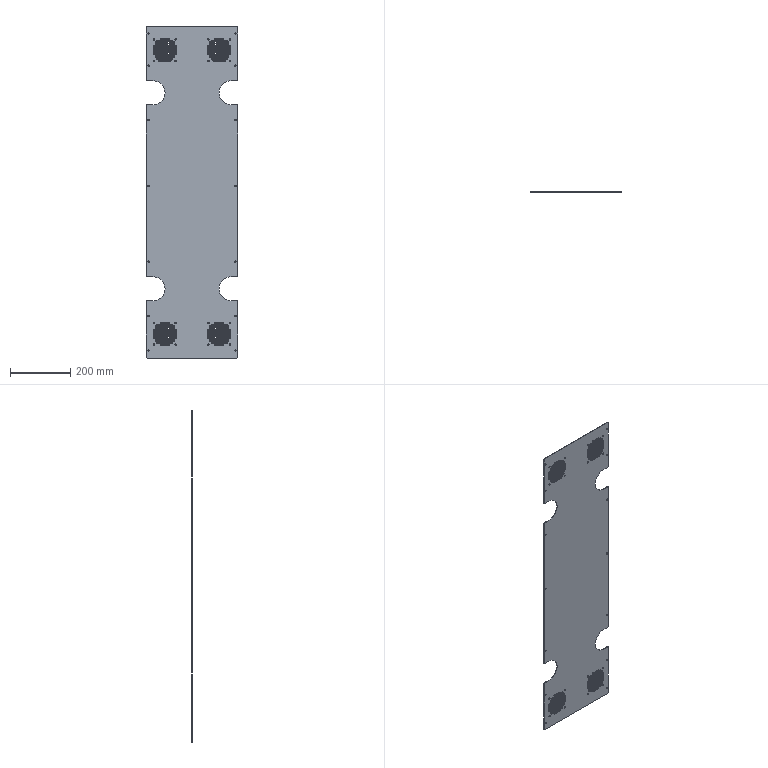Part | STEP file | 1519-2.stp.STEP | 1 solid | 1192 faces | box 302 x 2.5 x 1101 mm | volume 760439 mm3 | cylinder 1170 | plane 22 | commonest cylinder face diameters 5 x1136 4.5 x28 80 x6